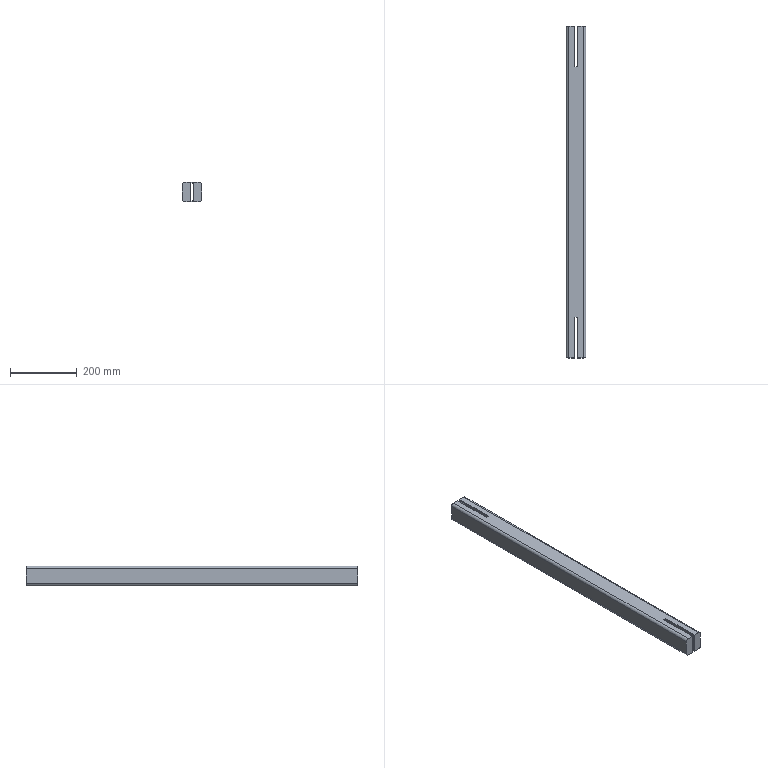Part | SolidWorks | features ICE 3, Extrusion 1 | 1 solid | 32 faces | box 60 x 998 x 60 mm | volume 853297 mm3 | plane 24 | cylinder 8 | commonest cylinder face diameters 8 x4 16 x4
STEP:
#1=CARTESIAN_POINT('',(22.,998.,-30.));
#2=VERTEX_POINT('',#1);
#3=CARTESIAN_POINT('',(4.5,998.,-30.));
#4=VERTEX_POINT('',#3);
#5=CARTESIAN_POINT('',(-22.,998.,-30.));
#6=DIRECTION('',(-1.,0.,0.));
#7=VECTOR('',#6,1000.);
#8=LINE('',#5,#7);
#9=EDGE_CURVE('',#2,#4,#8,.T.);
#10=ORIENTED_EDGE('',*,*,#9,.T.);
#11=CARTESIAN_POINT('',(4.5,998.,30.));
#12=VERTEX_POINT('',#11);
#13=CARTESIAN_POINT('',(4.5,998.,22.));
#14=DIRECTION('',(0.,0.,1.));
#15=VECTOR('',#14,1000.);
#16=LINE('',#13,#15);
#17=EDGE_CURVE('',#4,#12,#16,.T.);
#18=ORIENTED_EDGE('',*,*,#17,.T.);
#19=CARTESIAN_POINT('',(22.,998.,30.));
#20=VERTEX_POINT('',#19);
#21=CARTESIAN_POINT('',(-22.,998.,30.));
#22=DIRECTION('',(1.,0.,0.));
#23=VECTOR('',#22,1000.);
#24=LINE('',#21,#23);
#25=EDGE_CURVE('',#12,#20,#24,.T.);
#26=ORIENTED_EDGE('',*,*,#25,.T.);
#27=CARTESIAN_POINT('',(30.,998.,22.));
#28=VERTEX_POINT('',#27);
#29=CARTESIAN_POINT('',(22.,998.,22.));
#30=DIRECTION('',(0.,1.,0.));
#31=DIRECTION('',(0.,0.,1.));
#32=AXIS2_PLACEMENT_3D('',#29,#30,#31);
#33=CIRCLE('',#32,8.);
#34=EDGE_CURVE('',#20,#28,#33,.T.);
#35=ORIENTED_EDGE('',*,*,#34,.T.);
#36=CARTESIAN_POINT('',(30.,998.,-22.));
#37=VERTEX_POINT('',#36);
#38=CARTESIAN_POINT('',(30.,998.,22.));
#39=DIRECTION('',(0.,0.,-1.));
#40=VECTOR('',#39,1000.);
#41=LINE('',#38,#40);
#42=EDGE_CURVE('',#28,#37,#41,.T.);
#43=ORIENTED_EDGE('',*,*,#42,.T.);
#44=CARTESIAN_POINT('',(22.,998.,-22.));
#45=DIRECTION('',(0.,1.,0.));
#46=DIRECTION('',(0.,0.,-1.));
#47=AXIS2_PLACEMENT_3D('',#44,#45,#46);
#48=CIRCLE('',#47,8.);
#49=EDGE_CURVE('',#37,#2,#48,.T.);
#50=ORIENTED_EDGE('',*,*,#49,.T.);
#51=EDGE_LOOP('',(#10,#18,#26,#35,#43,#50));
#52=FACE_OUTER_BOUND('',#51,.T.);
#53=CARTESIAN_POINT('',(-22.,998.,22.));
#54=DIRECTION('',(0.,-1.,0.));
#55=DIRECTION('',(0.,0.,-1.));
#56=AXIS2_PLACEMENT_3D('',#53,#54,#55);
#57=PLANE('',#56);
#58=ADVANCED_FACE('',(#52),#57,.F.);
#59=CARTESIAN_POINT('',(4.5,0.,30.));
#60=VERTEX_POINT('',#59);
#61=CARTESIAN_POINT('',(22.,0.,30.));
#62=VERTEX_POINT('',#61);
#63=CARTESIAN_POINT('',(-22.,0.,30.));
#64=DIRECTION('',(1.,0.,0.));
#65=VECTOR('',#64,1000.);
#66=LINE('',#63,#65);
#67=EDGE_CURVE('',#60,#62,#66,.T.);
#68=ORIENTED_EDGE('',*,*,#67,.F.);
#69=CARTESIAN_POINT('',(4.5,0.,-30.));
#70=VERTEX_POINT('',#69);
#71=CARTESIAN_POINT('',(4.5,0.,22.));
#72=DIRECTION('',(0.,0.,1.));
#73=VECTOR('',#72,1000.);
#74=LINE('',#71,#73);
#75=EDGE_CURVE('',#70,#60,#74,.T.);
#76=ORIENTED_EDGE('',*,*,#75,.F.);
#77=CARTESIAN_POINT('',(22.,0.,-30.));
#78=VERTEX_POINT('',#77);
#79=CARTESIAN_POINT('',(-22.,0.,-30.));
#80=DIRECTION('',(-1.,0.,0.));
#81=VECTOR('',#80,1000.);
#82=LINE('',#79,#81);
#83=EDGE_CURVE('',#78,#70,#82,.T.);
#84=ORIENTED_EDGE('',*,*,#83,.F.);
#85=CARTESIAN_POINT('',(30.,0.,-22.));
#86=VERTEX_POINT('',#85);
#87=CARTESIAN_POINT('',(22.,0.,-22.));
#88=DIRECTION('',(0.,1.,0.));
#89=DIRECTION('',(0.,0.,-1.));
#90=AXIS2_PLACEMENT_3D('',#87,#88,#89);
#91=CIRCLE('',#90,8.);
#92=EDGE_CURVE('',#86,#78,#91,.T.);
#93=ORIENTED_EDGE('',*,*,#92,.F.);
#94=CARTESIAN_POINT('',(30.,0.,22.));
#95=VERTEX_POINT('',#94);
#96=CARTESIAN_POINT('',(30.,0.,22.));
#97=DIRECTION('',(0.,0.,-1.));
#98=VECTOR('',#97,1000.);
#99=LINE('',#96,#98);
#100=EDGE_CURVE('',#95,#86,#99,.T.);
#101=ORIENTED_EDGE('',*,*,#100,.F.);
#102=CARTESIAN_POINT('',(22.,0.,22.));
#103=DIRECTION('',(0.,1.,0.));
#104=DIRECTION('',(0.,0.,1.));
#105=AXIS2_PLACEMENT_3D('',#102,#103,#104);
#106=CIRCLE('',#105,8.);
#107=EDGE_CURVE('',#62,#95,#106,.T.);
#108=ORIENTED_EDGE('',*,*,#107,.F.);
#109=EDGE_LOOP('',(#68,#76,#84,#93,#101,#108));
#110=FACE_OUTER_BOUND('',#109,.T.);
#111=CARTESIAN_POINT('',(-22.,0.,22.));
#112=DIRECTION('',(0.,-1.,0.));
#113=DIRECTION('',(0.,0.,-1.));
#114=AXIS2_PLACEMENT_3D('',#111,#112,#113);
#115=PLANE('',#114);
#116=ADVANCED_FACE('',(#110),#115,.T.);
#117=CARTESIAN_POINT('',(-4.5,998.,30.));
#118=VERTEX_POINT('',#117);
#119=CARTESIAN_POINT('',(-4.5,998.,-30.));
#120=VERTEX_POINT('',#119);
#121=CARTESIAN_POINT('',(-4.5,998.,22.));
#122=DIRECTION('',(0.,0.,-1.));
#123=VECTOR('',#122,1000.);
#124=LINE('',#121,#123);
#125=EDGE_CURVE('',#118,#120,#124,.T.);
#126=ORIENTED_EDGE('',*,*,#125,.T.);
#127=CARTESIAN_POINT('',(-22.,998.,-30.));
#128=VERTEX_POINT('',#127);
#129=CARTESIAN_POINT('',(-22.,998.,-30.));
#130=DIRECTION('',(-1.,0.,0.));
#131=VECTOR('',#130,1000.);
#132=LINE('',#129,#131);
#133=EDGE_CURVE('',#120,#128,#132,.T.);
#134=ORIENTED_EDGE('',*,*,#133,.T.);
#135=CARTESIAN_POINT('',(-30.,998.,-22.));
#136=VERTEX_POINT('',#135);
#137=CARTESIAN_POINT('',(-22.,998.,-22.));
#138=DIRECTION('',(0.,1.,0.));
#139=DIRECTION('',(0.,0.,-1.));
#140=AXIS2_PLACEMENT_3D('',#137,#138,#139);
#141=CIRCLE('',#140,8.);
#142=EDGE_CURVE('',#128,#136,#141,.T.);
#143=ORIENTED_EDGE('',*,*,#142,.T.);
#144=CARTESIAN_POINT('',(-30.,998.,22.));
#145=VERTEX_POINT('',#144);
#146=CARTESIAN_POINT('',(-30.,998.,22.));
#147=DIRECTION('',(0.,0.,1.));
#148=VECTOR('',#147,1000.);
#149=LINE('',#146,#148);
#150=EDGE_CURVE('',#136,#145,#149,.T.);
#151=ORIENTED_EDGE('',*,*,#150,.T.);
#152=CARTESIAN_POINT('',(-22.,998.,30.));
#153=VERTEX_POINT('',#152);
#154=CARTESIAN_POINT('',(-22.,998.,22.));
#155=DIRECTION('',(0.,1.,0.));
#156=DIRECTION('',(0.,0.,-1.));
#157=AXIS2_PLACEMENT_3D('',#154,#155,#156);
#158=CIRCLE('',#157,8.);
#159=EDGE_CURVE('',#145,#153,#158,.T.);
#160=ORIENTED_EDGE('',*,*,#159,.T.);
#161=CARTESIAN_POINT('',(-22.,998.,30.));
#162=DIRECTION('',(1.,0.,0.));
#163=VECTOR('',#162,1000.);
#164=LINE('',#161,#163);
#165=EDGE_CURVE('',#153,#118,#164,.T.);
#166=ORIENTED_EDGE('',*,*,#165,.T.);
#167=EDGE_LOOP('',(#126,#134,#143,#151,#160,#166));
#168=FACE_OUTER_BOUND('',#167,.T.);
#169=CARTESIAN_POINT('',(-22.,998.,22.));
#170=DIRECTION('',(0.,-1.,0.));
#171=DIRECTION('',(0.,0.,-1.));
#172=AXIS2_PLACEMENT_3D('',#169,#170,#171);
#173=PLANE('',#172);
#174=ADVANCED_FACE('',(#168),#173,.F.);
#175=CARTESIAN_POINT('',(-4.5,0.,-30.));
#176=VERTEX_POINT('',#175);
#177=CARTESIAN_POINT('',(-22.,0.,-30.));
#178=VERTEX_POINT('',#177);
#179=CARTESIAN_POINT('',(-22.,0.,-30.));
#180=DIRECTION('',(-1.,0.,0.));
#181=VECTOR('',#180,1000.);
#182=LINE('',#179,#181);
#183=EDGE_CURVE('',#176,#178,#182,.T.);
#184=ORIENTED_EDGE('',*,*,#183,.F.);
#185=CARTESIAN_POINT('',(-4.5,0.,30.));
#186=VERTEX_POINT('',#185);
#187=CARTESIAN_POINT('',(-4.5,0.,22.));
#188=DIRECTION('',(0.,0.,-1.));
#189=VECTOR('',#188,1000.);
#190=LINE('',#187,#189);
#191=EDGE_CURVE('',#186,#176,#190,.T.);
#192=ORIENTED_EDGE('',*,*,#191,.F.);
#193=CARTESIAN_POINT('',(-22.,0.,30.));
#194=VERTEX_POINT('',#193);
#195=CARTESIAN_POINT('',(-22.,0.,30.));
#196=DIRECTION('',(1.,0.,0.));
#197=VECTOR('',#196,1000.);
#198=LINE('',#195,#197);
#199=EDGE_CURVE('',#194,#186,#198,.T.);
#200=ORIENTED_EDGE('',*,*,#199,.F.);
#201=CARTESIAN_POINT('',(-30.,0.,22.));
#202=VERTEX_POINT('',#201);
#203=CARTESIAN_POINT('',(-22.,0.,22.));
#204=DIRECTION('',(0.,1.,0.));
#205=DIRECTION('',(0.,0.,-1.));
#206=AXIS2_PLACEMENT_3D('',#203,#204,#205);
#207=CIRCLE('',#206,8.);
#208=EDGE_CURVE('',#202,#194,#207,.T.);
#209=ORIENTED_EDGE('',*,*,#208,.F.);
#210=CARTESIAN_POINT('',(-30.,0.,-22.));
#211=VERTEX_POINT('',#210);
#212=CARTESIAN_POINT('',(-30.,0.,22.));
#213=DIRECTION('',(0.,0.,1.));
#214=VECTOR('',#213,1000.);
#215=LINE('',#212,#214);
#216=EDGE_CURVE('',#211,#202,#215,.T.);
#217=ORIENTED_EDGE('',*,*,#216,.F.);
#218=CARTESIAN_POINT('',(-22.,0.,-22.));
#219=DIRECTION('',(0.,1.,0.));
#220=DIRECTION('',(0.,0.,-1.));
#221=AXIS2_PLACEMENT_3D('',#218,#219,#220);
#222=CIRCLE('',#221,8.);
#223=EDGE_CURVE('',#178,#211,#222,.T.);
#224=ORIENTED_EDGE('',*,*,#223,.F.);
#225=EDGE_LOOP('',(#184,#192,#200,#209,#217,#224));
#226=FACE_OUTER_BOUND('',#225,.T.);
#227=CARTESIAN_POINT('',(-22.,0.,22.));
#228=DIRECTION('',(0.,-1.,0.));
#229=DIRECTION('',(0.,0.,-1.));
#230=AXIS2_PLACEMENT_3D('',#227,#228,#229);
#231=PLANE('',#230);
#232=ADVANCED_FACE('',(#226),#231,.T.);
#233=ORIENTED_EDGE('',*,*,#208,.T.);
#234=CARTESIAN_POINT('',(-22.,998.,30.));
#235=DIRECTION('',(0.,-1.,0.));
#236=VECTOR('',#235,1000.);
#237=LINE('',#234,#236);
#238=EDGE_CURVE('',#153,#194,#237,.T.);
#239=ORIENTED_EDGE('',*,*,#238,.F.);
#240=ORIENTED_EDGE('',*,*,#159,.F.);
#241=CARTESIAN_POINT('',(-30.,998.,22.));
#242=DIRECTION('',(0.,-1.,0.));
#243=VECTOR('',#242,1000.);
#244=LINE('',#241,#243);
#245=EDGE_CURVE('',#145,#202,#244,.T.);
#246=ORIENTED_EDGE('',*,*,#245,.T.);
#247=EDGE_LOOP('',(#233,#239,#240,#246));
#248=FACE_OUTER_BOUND('',#247,.T.);
#249=CARTESIAN_POINT('',(-22.,998.,22.));
#250=DIRECTION('',(0.,-1.,0.));
#251=DIRECTION('',(0.,0.,-1.));
#252=AXIS2_PLACEMENT_3D('',#249,#250,#251);
#253=CYLINDRICAL_SURFACE('',#252,8.);
#254=ADVANCED_FACE('',(#248),#253,.T.);
#255=ORIENTED_EDGE('',*,*,#25,.F.);
#256=CARTESIAN_POINT('',(4.5,876.,30.));
#257=VERTEX_POINT('',#256);
#258=CARTESIAN_POINT('',(4.5,998.,30.));
#259=DIRECTION('',(0.,-1.,0.));
#260=VECTOR('',#259,1000.);
#261=LINE('',#258,#260);
#262=EDGE_CURVE('',#12,#257,#261,.T.);
#263=ORIENTED_EDGE('',*,*,#262,.T.);
#264=CARTESIAN_POINT('',(-4.5,876.,30.));
#265=VERTEX_POINT('',#264);
#266=CARTESIAN_POINT('',(-22.,876.,30.));
#267=DIRECTION('',(-1.,0.,0.));
#268=VECTOR('',#267,1000.);
#269=LINE('',#266,#268);
#270=EDGE_CURVE('',#257,#265,#269,.T.);
#271=ORIENTED_EDGE('',*,*,#270,.T.);
#272=CARTESIAN_POINT('',(-4.5,998.,30.));
#273=DIRECTION('',(0.,1.,0.));
#274=VECTOR('',#273,1000.);
#275=LINE('',#272,#274);
#276=EDGE_CURVE('',#265,#118,#275,.T.);
#277=ORIENTED_EDGE('',*,*,#276,.T.);
#278=ORIENTED_EDGE('',*,*,#165,.F.);
#279=ORIENTED_EDGE('',*,*,#238,.T.);
#280=ORIENTED_EDGE('',*,*,#199,.T.);
#281=CARTESIAN_POINT('',(-4.5,122.,30.));
#282=VERTEX_POINT('',#281);
#283=CARTESIAN_POINT('',(-4.5,998.,30.));
#284=DIRECTION('',(0.,1.,0.));
#285=VECTOR('',#284,1000.);
#286=LINE('',#283,#285);
#287=EDGE_CURVE('',#186,#282,#286,.T.);
#288=ORIENTED_EDGE('',*,*,#287,.T.);
#289=CARTESIAN_POINT('',(4.5,122.,30.));
#290=VERTEX_POINT('',#289);
#291=CARTESIAN_POINT('',(-22.,122.,30.));
#292=DIRECTION('',(1.,0.,0.));
#293=VECTOR('',#292,1000.);
#294=LINE('',#291,#293);
#295=EDGE_CURVE('',#282,#290,#294,.T.);
#296=ORIENTED_EDGE('',*,*,#295,.T.);
#297=CARTESIAN_POINT('',(4.5,998.,30.));
#298=DIRECTION('',(0.,-1.,0.));
#299=VECTOR('',#298,1000.);
#300=LINE('',#297,#299);
#301=EDGE_CURVE('',#290,#60,#300,.T.);
#302=ORIENTED_EDGE('',*,*,#301,.T.);
#303=ORIENTED_EDGE('',*,*,#67,.T.);
#304=CARTESIAN_POINT('',(22.,998.,30.));
#305=DIRECTION('',(0.,-1.,0.));
#306=VECTOR('',#305,1000.);
#307=LINE('',#304,#306);
#308=EDGE_CURVE('',#20,#62,#307,.T.);
#309=ORIENTED_EDGE('',*,*,#308,.F.);
#310=EDGE_LOOP('',(#255,#263,#271,#277,#278,#279,#280,#288,#296,#302,#303,#309));
#311=FACE_OUTER_BOUND('',#310,.T.);
#312=CARTESIAN_POINT('',(-22.,998.,30.));
#313=DIRECTION('',(0.,0.,-1.));
#314=DIRECTION('',(-1.,0.,0.));
#315=AXIS2_PLACEMENT_3D('',#312,#313,#314);
#316=PLANE('',#315);
#317=ADVANCED_FACE('',(#311),#316,.F.);
#318=ORIENTED_EDGE('',*,*,#107,.T.);
#319=CARTESIAN_POINT('',(30.,998.,22.));
#320=DIRECTION('',(0.,-1.,0.));
#321=VECTOR('',#320,1000.);
#322=LINE('',#319,#321);
#323=EDGE_CURVE('',#28,#95,#322,.T.);
#324=ORIENTED_EDGE('',*,*,#323,.F.);
#325=ORIENTED_EDGE('',*,*,#34,.F.);
#326=ORIENTED_EDGE('',*,*,#308,.T.);
#327=EDGE_LOOP('',(#318,#324,#325,#326));
#328=FACE_OUTER_BOUND('',#327,.T.);
#329=CARTESIAN_POINT('',(22.,998.,22.));
#330=DIRECTION('',(0.,-1.,0.));
#331=DIRECTION('',(0.,0.,-1.));
#332=AXIS2_PLACEMENT_3D('',#329,#330,#331);
#333=CYLINDRICAL_SURFACE('',#332,8.);
#334=ADVANCED_FACE('',(#328),#333,.T.);
#335=ORIENTED_EDGE('',*,*,#100,.T.);
#336=CARTESIAN_POINT('',(30.,998.,-22.));
#337=DIRECTION('',(0.,-1.,0.));
#338=VECTOR('',#337,1000.);
#339=LINE('',#336,#338);
#340=EDGE_CURVE('',#37,#86,#339,.T.);
#341=ORIENTED_EDGE('',*,*,#340,.F.);
#342=ORIENTED_EDGE('',*,*,#42,.F.);
#343=ORIENTED_EDGE('',*,*,#323,.T.);
#344=EDGE_LOOP('',(#335,#341,#342,#343));
#345=FACE_OUTER_BOUND('',#344,.T.);
#346=CARTESIAN_POINT('',(30.,998.,22.));
#347=DIRECTION('',(-1.,0.,0.));
#348=DIRECTION('',(0.,0.,1.));
#349=AXIS2_PLACEMENT_3D('',#346,#347,#348);
#350=PLANE('',#349);
#351=ADVANCED_FACE('',(#345),#350,.F.);
#352=ORIENTED_EDGE('',*,*,#92,.T.);
#353=CARTESIAN_POINT('',(22.,998.,-30.));
#354=DIRECTION('',(0.,-1.,0.));
#355=VECTOR('',#354,1000.);
#356=LINE('',#353,#355);
#357=EDGE_CURVE('',#2,#78,#356,.T.);
#358=ORIENTED_EDGE('',*,*,#357,.F.);
#359=ORIENTED_EDGE('',*,*,#49,.F.);
#360=ORIENTED_EDGE('',*,*,#340,.T.);
#361=EDGE_LOOP('',(#352,#358,#359,#360));
#362=FACE_OUTER_BOUND('',#361,.T.);
#363=CARTESIAN_POINT('',(22.,998.,-22.));
#364=DIRECTION('',(0.,-1.,0.));
#365=DIRECTION('',(0.,0.,-1.));
#366=AXIS2_PLACEMENT_3D('',#363,#364,#365);
#367=CYLINDRICAL_SURFACE('',#366,8.);
#368=ADVANCED_FACE('',(#362),#367,.T.);
#369=CARTESIAN_POINT('',(-4.5,876.,-30.));
#370=VERTEX_POINT('',#369);
#371=CARTESIAN_POINT('',(4.5,876.,-30.));
#372=VERTEX_POINT('',#371);
#373=CARTESIAN_POINT('',(-4.5,876.,-30.));
#374=DIRECTION('',(1.,0.,0.));
#375=VECTOR('',#374,1000.);
#376=LINE('',#373,#375);
#377=EDGE_CURVE('',#370,#372,#376,.T.);
#378=ORIENTED_EDGE('',*,*,#377,.T.);
#379=CARTESIAN_POINT('',(4.5,1120.,-30.));
#380=DIRECTION('',(0.,1.,0.));
#381=VECTOR('',#380,1000.);
#382=LINE('',#379,#381);
#383=EDGE_CURVE('',#372,#4,#382,.T.);
#384=ORIENTED_EDGE('',*,*,#383,.T.);
#385=ORIENTED_EDGE('',*,*,#9,.F.);
#386=ORIENTED_EDGE('',*,*,#357,.T.);
#387=ORIENTED_EDGE('',*,*,#83,.T.);
#388=CARTESIAN_POINT('',(4.5,122.,-30.));
#389=VERTEX_POINT('',#388);
#390=CARTESIAN_POINT('',(4.5,-122.,-30.));
#391=DIRECTION('',(0.,1.,0.));
#392=VECTOR('',#391,1000.);
#393=LINE('',#390,#392);
#394=EDGE_CURVE('',#70,#389,#393,.T.);
#395=ORIENTED_EDGE('',*,*,#394,.T.);
#396=CARTESIAN_POINT('',(-4.5,122.,-30.));
#397=VERTEX_POINT('',#396);
#398=CARTESIAN_POINT('',(-4.5,122.,-30.));
#399=DIRECTION('',(-1.,0.,0.));
#400=VECTOR('',#399,1000.);
#401=LINE('',#398,#400);
#402=EDGE_CURVE('',#389,#397,#401,.T.);
#403=ORIENTED_EDGE('',*,*,#402,.T.);
#404=CARTESIAN_POINT('',(-4.5,-122.,-30.));
#405=DIRECTION('',(0.,-1.,0.));
#406=VECTOR('',#405,1000.);
#407=LINE('',#404,#406);
#408=EDGE_CURVE('',#397,#176,#407,.T.);
#409=ORIENTED_EDGE('',*,*,#408,.T.);
#410=ORIENTED_EDGE('',*,*,#183,.T.);
#411=CARTESIAN_POINT('',(-22.,998.,-30.));
#412=DIRECTION('',(0.,-1.,0.));
#413=VECTOR('',#412,1000.);
#414=LINE('',#411,#413);
#415=EDGE_CURVE('',#128,#178,#414,.T.);
#416=ORIENTED_EDGE('',*,*,#415,.F.);
#417=ORIENTED_EDGE('',*,*,#133,.F.);
#418=CARTESIAN_POINT('',(-4.5,1120.,-30.));
#419=DIRECTION('',(0.,-1.,0.));
#420=VECTOR('',#419,1000.);
#421=LINE('',#418,#420);
#422=EDGE_CURVE('',#120,#370,#421,.T.);
#423=ORIENTED_EDGE('',*,*,#422,.T.);
#424=EDGE_LOOP('',(#378,#384,#385,#386,#387,#395,#403,#409,#410,#416,#417,#423));
#425=FACE_OUTER_BOUND('',#424,.T.);
#426=CARTESIAN_POINT('',(-22.,998.,-30.));
#427=DIRECTION('',(0.,0.,1.));
#428=DIRECTION('',(1.,0.,0.));
#429=AXIS2_PLACEMENT_3D('',#426,#427,#428);
#430=PLANE('',#429);
#431=ADVANCED_FACE('',(#425),#430,.F.);
#432=ORIENTED_EDGE('',*,*,#223,.T.);
#433=CARTESIAN_POINT('',(-30.,998.,-22.));
#434=DIRECTION('',(0.,-1.,0.));
#435=VECTOR('',#434,1000.);
#436=LINE('',#433,#435);
#437=EDGE_CURVE('',#136,#211,#436,.T.);
#438=ORIENTED_EDGE('',*,*,#437,.F.);
#439=ORIENTED_EDGE('',*,*,#142,.F.);
#440=ORIENTED_EDGE('',*,*,#415,.T.);
#441=EDGE_LOOP('',(#432,#438,#439,#440));
#442=FACE_OUTER_BOUND('',#441,.T.);
#443=CARTESIAN_POINT('',(-22.,998.,-22.));
#444=DIRECTION('',(0.,-1.,0.));
#445=DIRECTION('',(0.,0.,-1.));
#446=AXIS2_PLACEMENT_3D('',#443,#444,#445);
#447=CYLINDRICAL_SURFACE('',#446,8.);
#448=ADVANCED_FACE('',(#442),#447,.T.);
#449=ORIENTED_EDGE('',*,*,#216,.T.);
#450=ORIENTED_EDGE('',*,*,#245,.F.);
#451=ORIENTED_EDGE('',*,*,#150,.F.);
#452=ORIENTED_EDGE('',*,*,#437,.T.);
#453=EDGE_LOOP('',(#449,#450,#451,#452));
#454=FACE_OUTER_BOUND('',#453,.T.);
#455=CARTESIAN_POINT('',(-30.,998.,22.));
#456=DIRECTION('',(1.,0.,0.));
#457=DIRECTION('',(0.,0.,-1.));
#458=AXIS2_PLACEMENT_3D('',#455,#456,#457);
#459=PLANE('',#458);
#460=ADVANCED_FACE('',(#454),#459,.F.);
#461=CARTESIAN_POINT('',(-22.,4.,-26.));
#462=VERTEX_POINT('',#461);
#463=CARTESIAN_POINT('',(-26.,4.,-22.));
#464=VERTEX_POINT('',#463);
#465=CARTESIAN_POINT('',(-22.,4.,-22.));
#466=DIRECTION('',(0.,1.,0.));
#467=DIRECTION('',(0.,0.,1.));
#468=AXIS2_PLACEMENT_3D('',#465,#466,#467);
#469=CIRCLE('',#468,4.);
#470=EDGE_CURVE('',#462,#464,#469,.T.);
#471=ORIENTED_EDGE('',*,*,#470,.F.);
#472=CARTESIAN_POINT('',(-22.,994.,-26.));
#473=VERTEX_POINT('',#472);
#474=CARTESIAN_POINT('',(-22.,998.,-26.));
#475=DIRECTION('',(0.,-1.,0.));
#476=VECTOR('',#475,1000.);
#477=LINE('',#474,#476);
#478=EDGE_CURVE('',#473,#462,#477,.T.);
#479=ORIENTED_EDGE('',*,*,#478,.F.);
#480=CARTESIAN_POINT('',(-26.,994.,-22.));
#481=VERTEX_POINT('',#480);
#482=CARTESIAN_POINT('',(-22.,994.,-22.));
#483=DIRECTION('',(0.,-1.,0.));
#484=DIRECTION('',(0.,0.,-1.));
#485=AXIS2_PLACEMENT_3D('',#482,#483,#484);
#486=CIRCLE('',#485,4.);
#487=EDGE_CURVE('',#481,#473,#486,.T.);
#488=ORIENTED_EDGE('',*,*,#487,.F.);
#489=CARTESIAN_POINT('',(-26.,998.,-22.));
#490=DIRECTION('',(0.,-1.,0.));
#491=VECTOR('',#490,1000.);
#492=LINE('',#489,#491);
#493=EDGE_CURVE('',#481,#464,#492,.T.);
#494=ORIENTED_EDGE('',*,*,#493,.T.);
#495=EDGE_LOOP('',(#471,#479,#488,#494));
#496=FACE_OUTER_BOUND('',#495,.T.);
#497=CARTESIAN_POINT('',(-22.,998.,-22.));
#498=DIRECTION('',(0.,-1.,0.));
#499=DIRECTION('',(0.,0.,-1.));
#500=AXIS2_PLACEMENT_3D('',#497,#498,#499);
#501=CYLINDRICAL_SURFACE('',#500,4.);
#502=ADVANCED_FACE('',(#496),#501,.F.);
#503=CARTESIAN_POINT('',(-26.,4.,22.));
#504=VERTEX_POINT('',#503);
#505=CARTESIAN_POINT('',(-26.,4.,26.));
#506=DIRECTION('',(0.,0.,-1.));
#507=VECTOR('',#506,1000.);
#508=LINE('',#505,#507);
#509=EDGE_CURVE('',#504,#464,#508,.T.);
#510=ORIENTED_EDGE('',*,*,#509,.T.);
#511=ORIENTED_EDGE('',*,*,#493,.F.);
#512=CARTESIAN_POINT('',(-26.,994.,22.));
#513=VERTEX_POINT('',#512);
#514=CARTESIAN_POINT('',(-26.,994.,-26.));
#515=DIRECTION('',(0.,0.,1.));
#516=VECTOR('',#515,1000.);
#517=LINE('',#514,#516);
#518=EDGE_CURVE('',#481,#513,#517,.T.);
#519=ORIENTED_EDGE('',*,*,#518,.T.);
#520=CARTESIAN_POINT('',(-26.,998.,22.));
#521=DIRECTION('',(0.,-1.,0.));
#522=VECTOR('',#521,1000.);
#523=LINE('',#520,#522);
#524=EDGE_CURVE('',#513,#504,#523,.T.);
#525=ORIENTED_EDGE('',*,*,#524,.T.);
#526=EDGE_LOOP('',(#510,#511,#519,#525));
#527=FACE_OUTER_BOUND('',#526,.T.);
#528=CARTESIAN_POINT('',(-26.,998.,22.));
#529=DIRECTION('',(1.,0.,0.));
#530=DIRECTION('',(0.,0.,-1.));
#531=AXIS2_PLACEMENT_3D('',#528,#529,#530);
#532=PLANE('',#531);
#533=ADVANCED_FACE('',(#527),#532,.T.);
#534=CARTESIAN_POINT('',(-22.,4.,26.));
#535=VERTEX_POINT('',#534);
#536=CARTESIAN_POINT('',(-22.,4.,22.));
#537=DIRECTION('',(0.,1.,0.));
#538=DIRECTION('',(0.,0.,1.));
#539=AXIS2_PLACEMENT_3D('',#536,#537,#538);
#540=CIRCLE('',#539,4.);
#541=EDGE_CURVE('',#504,#535,#540,.T.);
#542=ORIENTED_EDGE('',*,*,#541,.F.);
#543=ORIENTED_EDGE('',*,*,#524,.F.);
#544=CARTESIAN_POINT('',(-22.,994.,26.));
#545=VERTEX_POINT('',#544);
#546=CARTESIAN_POINT('',(-22.,994.,22.));
#547=DIRECTION('',(0.,-1.,0.));
#548=DIRECTION('',(0.,0.,-1.));
#549=AXIS2_PLACEMENT_3D('',#546,#547,#548);
#550=CIRCLE('',#549,4.);
#551=EDGE_CURVE('',#545,#513,#550,.T.);
#552=ORIENTED_EDGE('',*,*,#551,.F.);
#553=CARTESIAN_POINT('',(-22.,998.,26.));
#554=DIRECTION('',(0.,-1.,0.));
#555=VECTOR('',#554,1000.);
#556=LINE('',#553,#555);
#557=EDGE_CURVE('',#545,#535,#556,.T.);
#558=ORIENTED_EDGE('',*,*,#557,.T.);
#559=EDGE_LOOP('',(#542,#543,#552,#558));
#560=FACE_OUTER_BOUND('',#559,.T.);
#561=CARTESIAN_POINT('',(-22.,998.,22.));
#562=DIRECTION('',(0.,-1.,0.));
#563=DIRECTION('',(0.,0.,-1.));
#564=AXIS2_PLACEMENT_3D('',#561,#562,#563);
#565=CYLINDRICAL_SURFACE('',#564,4.);
#566=ADVANCED_FACE('',(#560),#565,.F.);
#567=CARTESIAN_POINT('',(22.,4.,26.));
#568=VERTEX_POINT('',#567);
#569=CARTESIAN_POINT('',(4.5,4.,26.));
#570=VERTEX_POINT('',#569);
#571=CARTESIAN_POINT('',(4.5,4.,26.));
#572=DIRECTION('',(-1.,0.,0.));
#573=VECTOR('',#572,1000.);
#574=LINE('',#571,#573);
#575=EDGE_CURVE('',#568,#570,#574,.T.);
#576=ORIENTED_EDGE('',*,*,#575,.T.);
#577=CARTESIAN_POINT('',(4.5,122.,26.));
#578=VERTEX_POINT('',#577);
#579=CARTESIAN_POINT('',(4.5,998.,26.));
#580=DIRECTION('',(0.,-1.,0.));
#581=VECTOR('',#580,1000.);
#582=LINE('',#579,#581);
#583=EDGE_CURVE('',#578,#570,#582,.T.);
#584=ORIENTED_EDGE('',*,*,#583,.F.);
#585=CARTESIAN_POINT('',(-4.5,122.,26.));
#586=VERTEX_POINT('',#585);
#587=CARTESIAN_POINT('',(-22.,122.,26.));
#588=DIRECTION('',(1.,0.,0.));
#589=VECTOR('',#588,1000.);
#590=LINE('',#587,#589);
#591=EDGE_CURVE('',#586,#578,#590,.T.);
#592=ORIENTED_EDGE('',*,*,#591,.F.);
#593=CARTESIAN_POINT('',(-4.5,4.,26.));
#594=VERTEX_POINT('',#593);
#595=CARTESIAN_POINT('',(-4.5,998.,26.));
#596=DIRECTION('',(0.,1.,0.));
#597=VECTOR('',#596,1000.);
#598=LINE('',#595,#597);
#599=EDGE_CURVE('',#594,#586,#598,.T.);
#600=ORIENTED_EDGE('',*,*,#599,.F.);
#601=CARTESIAN_POINT('',(-4.5,4.,26.));
#602=DIRECTION('',(-1.,0.,0.));
#603=VECTOR('',#602,1000.);
#604=LINE('',#601,#603);
#605=EDGE_CURVE('',#594,#535,#604,.T.);
#606=ORIENTED_EDGE('',*,*,#605,.T.);
#607=ORIENTED_EDGE('',*,*,#557,.F.);
#608=CARTESIAN_POINT('',(-4.5,994.,26.));
#609=VERTEX_POINT('',#608);
#610=CARTESIAN_POINT('',(-4.5,994.,26.));
#611=DIRECTION('',(1.,0.,0.));
#612=VECTOR('',#611,1000.);
#613=LINE('',#610,#612);
#614=EDGE_CURVE('',#545,#609,#613,.T.);
#615=ORIENTED_EDGE('',*,*,#614,.T.);
#616=CARTESIAN_POINT('',(-4.5,876.,26.));
#617=VERTEX_POINT('',#616);
#618=CARTESIAN_POINT('',(-4.5,998.,26.));
#619=DIRECTION('',(0.,1.,0.));
#620=VECTOR('',#619,1000.);
#621=LINE('',#618,#620);
#622=EDGE_CURVE('',#617,#609,#621,.T.);
#623=ORIENTED_EDGE('',*,*,#622,.F.);
#624=CARTESIAN_POINT('',(4.5,876.,26.));
#625=VERTEX_POINT('',#624);
#626=CARTESIAN_POINT('',(-22.,876.,26.));
#627=DIRECTION('',(-1.,0.,0.));
#628=VECTOR('',#627,1000.);
#629=LINE('',#626,#628);
#630=EDGE_CURVE('',#625,#617,#629,.T.);
#631=ORIENTED_EDGE('',*,*,#630,.F.);
#632=CARTESIAN_POINT('',(4.5,994.,26.));
#633=VERTEX_POINT('',#632);
#634=CARTESIAN_POINT('',(4.5,998.,26.));
#635=DIRECTION('',(0.,-1.,0.));
#636=VECTOR('',#635,1000.);
#637=LINE('',#634,#636);
#638=EDGE_CURVE('',#633,#625,#637,.T.);
#639=ORIENTED_EDGE('',*,*,#638,.F.);
#640=CARTESIAN_POINT('',(22.,994.,26.));
#641=VERTEX_POINT('',#640);
#642=CARTESIAN_POINT('',(4.5,994.,26.));
#643=DIRECTION('',(1.,0.,0.));
#644=VECTOR('',#643,1000.);
#645=LINE('',#642,#644);
#646=EDGE_CURVE('',#633,#641,#645,.T.);
#647=ORIENTED_EDGE('',*,*,#646,.T.);
#648=CARTESIAN_POINT('',(22.,998.,26.));
#649=DIRECTION('',(0.,-1.,0.));
#650=VECTOR('',#649,1000.);
#651=LINE('',#648,#650);
#652=EDGE_CURVE('',#641,#568,#651,.T.);
#653=ORIENTED_EDGE('',*,*,#652,.T.);
#654=EDGE_LOOP('',(#576,#584,#592,#600,#606,#607,#615,#623,#631,#639,#647,#653));
#655=FACE_OUTER_BOUND('',#654,.T.);
#656=CARTESIAN_POINT('',(-22.,998.,26.));
#657=DIRECTION('',(0.,0.,-1.));
#658=DIRECTION('',(-1.,0.,0.));
#659=AXIS2_PLACEMENT_3D('',#656,#657,#658);
#660=PLANE('',#659);
#661=ADVANCED_FACE('',(#655),#660,.T.);
#662=CARTESIAN_POINT('',(26.,4.,22.));
#663=VERTEX_POINT('',#662);
#664=CARTESIAN_POINT('',(22.,4.,22.));
#665=DIRECTION('',(0.,1.,0.));
#666=DIRECTION('',(0.,0.,1.));
#667=AXIS2_PLACEMENT_3D('',#664,#665,#666);
#668=CIRCLE('',#667,4.);
#669=EDGE_CURVE('',#568,#663,#668,.T.);
#670=ORIENTED_EDGE('',*,*,#669,.F.);
#671=ORIENTED_EDGE('',*,*,#652,.F.);
#672=CARTESIAN_POINT('',(26.,994.,22.));
#673=VERTEX_POINT('',#672);
#674=CARTESIAN_POINT('',(22.,994.,22.));
#675=DIRECTION('',(0.,-1.,0.));
#676=DIRECTION('',(0.,0.,-1.));
#677=AXIS2_PLACEMENT_3D('',#674,#675,#676);
#678=CIRCLE('',#677,4.);
#679=EDGE_CURVE('',#673,#641,#678,.T.);
#680=ORIENTED_EDGE('',*,*,#679,.F.);
#681=CARTESIAN_POINT('',(26.,998.,22.));
#682=DIRECTION('',(0.,-1.,0.));
#683=VECTOR('',#682,1000.);
#684=LINE('',#681,#683);
#685=EDGE_CURVE('',#673,#663,#684,.T.);
#686=ORIENTED_EDGE('',*,*,#685,.T.);
#687=EDGE_LOOP('',(#670,#671,#680,#686));
#688=FACE_OUTER_BOUND('',#687,.T.);
#689=CARTESIAN_POINT('',(22.,998.,22.));
#690=DIRECTION('',(0.,-1.,0.));
#691=DIRECTION('',(0.,0.,-1.));
#692=AXIS2_PLACEMENT_3D('',#689,#690,#691);
#693=CYLINDRICAL_SURFACE('',#692,4.);
#694=ADVANCED_FACE('',(#688),#693,.F.);
#695=CARTESIAN_POINT('',(26.,4.,-22.));
#696=VERTEX_POINT('',#695);
#697=CARTESIAN_POINT('',(26.,4.,26.));
#698=DIRECTION('',(0.,0.,1.));
#699=VECTOR('',#698,1000.);
#700=LINE('',#697,#699);
#701=EDGE_CURVE('',#696,#663,#700,.T.);
#702=ORIENTED_EDGE('',*,*,#701,.T.);
#703=ORIENTED_EDGE('',*,*,#685,.F.);
#704=CARTESIAN_POINT('',(26.,994.,-22.));
#705=VERTEX_POINT('',#704);
#706=CARTESIAN_POINT('',(26.,994.,-26.));
#707=DIRECTION('',(0.,0.,-1.));
#708=VECTOR('',#707,1000.);
#709=LINE('',#706,#708);
#710=EDGE_CURVE('',#673,#705,#709,.T.);
#711=ORIENTED_EDGE('',*,*,#710,.T.);
#712=CARTESIAN_POINT('',(26.,998.,-22.));
#713=DIRECTION('',(0.,-1.,0.));
#714=VECTOR('',#713,1000.);
#715=LINE('',#712,#714);
#716=EDGE_CURVE('',#705,#696,#715,.T.);
#717=ORIENTED_EDGE('',*,*,#716,.T.);
#718=EDGE_LOOP('',(#702,#703,#711,#717));
#719=FACE_OUTER_BOUND('',#718,.T.);
#720=CARTESIAN_POINT('',(26.,998.,22.));
#721=DIRECTION('',(-1.,0.,0.));
#722=DIRECTION('',(0.,0.,1.));
#723=AXIS2_PLACEMENT_3D('',#720,#721,#722);
#724=PLANE('',#723);
#725=ADVANCED_FACE('',(#719),#724,.T.);
#726=CARTESIAN_POINT('',(22.,4.,-26.));
#727=VERTEX_POINT('',#726);
#728=CARTESIAN_POINT('',(22.,4.,-22.));
#729=DIRECTION('',(0.,1.,0.));
#730=DIRECTION('',(0.,0.,1.));
#731=AXIS2_PLACEMENT_3D('',#728,#729,#730);
#732=CIRCLE('',#731,4.);
#733=EDGE_CURVE('',#696,#727,#732,.T.);
#734=ORIENTED_EDGE('',*,*,#733,.F.);
#735=ORIENTED_EDGE('',*,*,#716,.F.);
#736=CARTESIAN_POINT('',(22.,994.,-26.));
#737=VERTEX_POINT('',#736);
#738=CARTESIAN_POINT('',(22.,994.,-22.));
#739=DIRECTION('',(0.,-1.,0.));
#740=DIRECTION('',(0.,0.,-1.));
#741=AXIS2_PLACEMENT_3D('',#738,#739,#740);
#742=CIRCLE('',#741,4.);
#743=EDGE_CURVE('',#737,#705,#742,.T.);
#744=ORIENTED_EDGE('',*,*,#743,.F.);
#745=CARTESIAN_POINT('',(22.,998.,-26.));
#746=DIRECTION('',(0.,-1.,0.));
#747=VECTOR('',#746,1000.);
#748=LINE('',#745,#747);
#749=EDGE_CURVE('',#737,#727,#748,.T.);
#750=ORIENTED_EDGE('',*,*,#749,.T.);
#751=EDGE_LOOP('',(#734,#735,#744,#750));
#752=FACE_OUTER_BOUND('',#751,.T.);
#753=CARTESIAN_POINT('',(22.,998.,-22.));
#754=DIRECTION('',(0.,-1.,0.));
#755=DIRECTION('',(0.,0.,-1.));
#756=AXIS2_PLACEMENT_3D('',#753,#754,#755);
#757=CYLINDRICAL_SURFACE('',#756,4.);
#758=ADVANCED_FACE('',(#752),#757,.F.);
#759=CARTESIAN_POINT('',(4.5,4.,-26.));
#760=VERTEX_POINT('',#759);
#761=CARTESIAN_POINT('',(4.5,4.,-26.));
#762=DIRECTION('',(1.,0.,0.));
#763=VECTOR('',#762,1000.);
#764=LINE('',#761,#763);
#765=EDGE_CURVE('',#760,#727,#764,.T.);
#766=ORIENTED_EDGE('',*,*,#765,.T.);
#767=ORIENTED_EDGE('',*,*,#749,.F.);
#768=CARTESIAN_POINT('',(4.5,994.,-26.));
#769=VERTEX_POINT('',#768);
#770=CARTESIAN_POINT('',(4.5,994.,-26.));
#771=DIRECTION('',(-1.,0.,0.));
#772=VECTOR('',#771,1000.);
#773=LINE('',#770,#772);
#774=EDGE_CURVE('',#737,#769,#773,.T.);
#775=ORIENTED_EDGE('',*,*,#774,.T.);
#776=CARTESIAN_POINT('',(4.5,876.,-26.));
#777=VERTEX_POINT('',#776);
#778=CARTESIAN_POINT('',(4.5,998.,-26.));
#779=DIRECTION('',(0.,1.,0.));
#780=VECTOR('',#779,1000.);
#781=LINE('',#778,#780);
#782=EDGE_CURVE('',#777,#769,#781,.T.);
#783=ORIENTED_EDGE('',*,*,#782,.F.);
#784=CARTESIAN_POINT('',(-4.5,876.,-26.));
#785=VERTEX_POINT('',#784);
#786=CARTESIAN_POINT('',(-22.,876.,-26.));
#787=DIRECTION('',(1.,0.,0.));
#788=VECTOR('',#787,1000.);
#789=LINE('',#786,#788);
#790=EDGE_CURVE('',#785,#777,#789,.T.);
#791=ORIENTED_EDGE('',*,*,#790,.F.);
#792=CARTESIAN_POINT('',(-4.5,994.,-26.));
#793=VERTEX_POINT('',#792);
#794=CARTESIAN_POINT('',(-4.5,998.,-26.));
#795=DIRECTION('',(0.,-1.,0.));
#796=VECTOR('',#795,1000.);
#797=LINE('',#794,#796);
#798=EDGE_CURVE('',#793,#785,#797,.T.);
#799=ORIENTED_EDGE('',*,*,#798,.F.);
#800=CARTESIAN_POINT('',(-4.5,994.,-26.));
#801=DIRECTION('',(-1.,0.,0.));
#802=VECTOR('',#801,1000.);
#803=LINE('',#800,#802);
#804=EDGE_CURVE('',#793,#473,#803,.T.);
#805=ORIENTED_EDGE('',*,*,#804,.T.);
#806=ORIENTED_EDGE('',*,*,#478,.T.);
#807=CARTESIAN_POINT('',(-4.5,4.,-26.));
#808=VERTEX_POINT('',#807);
#809=CARTESIAN_POINT('',(-4.5,4.,-26.));
#810=DIRECTION('',(1.,0.,0.));
#811=VECTOR('',#810,1000.);
#812=LINE('',#809,#811);
#813=EDGE_CURVE('',#462,#808,#812,.T.);
#814=ORIENTED_EDGE('',*,*,#813,.T.);
#815=CARTESIAN_POINT('',(-4.5,122.,-26.));
#816=VERTEX_POINT('',#815);
#817=CARTESIAN_POINT('',(-4.5,998.,-26.));
#818=DIRECTION('',(0.,-1.,0.));
#819=VECTOR('',#818,1000.);
#820=LINE('',#817,#819);
#821=EDGE_CURVE('',#816,#808,#820,.T.);
#822=ORIENTED_EDGE('',*,*,#821,.F.);
#823=CARTESIAN_POINT('',(4.5,122.,-26.));
#824=VERTEX_POINT('',#823);
#825=CARTESIAN_POINT('',(-22.,122.,-26.));
#826=DIRECTION('',(-1.,0.,0.));
#827=VECTOR('',#826,1000.);
#828=LINE('',#825,#827);
#829=EDGE_CURVE('',#824,#816,#828,.T.);
#830=ORIENTED_EDGE('',*,*,#829,.F.);
#831=CARTESIAN_POINT('',(4.5,998.,-26.));
#832=DIRECTION('',(0.,1.,0.));
#833=VECTOR('',#832,1000.);
#834=LINE('',#831,#833);
#835=EDGE_CURVE('',#760,#824,#834,.T.);
#836=ORIENTED_EDGE('',*,*,#835,.F.);
#837=EDGE_LOOP('',(#766,#767,#775,#783,#791,#799,#805,#806,#814,#822,#830,#836));
#838=FACE_OUTER_BOUND('',#837,.T.);
#839=CARTESIAN_POINT('',(-22.,998.,-26.));
#840=DIRECTION('',(0.,0.,1.));
#841=DIRECTION('',(1.,0.,0.));
#842=AXIS2_PLACEMENT_3D('',#839,#840,#841);
#843=PLANE('',#842);
#844=ADVANCED_FACE('',(#838),#843,.T.);
#845=ORIENTED_EDGE('',*,*,#829,.T.);
#846=CARTESIAN_POINT('',(-4.5,122.,-30.));
#847=DIRECTION('',(0.,0.,1.));
#848=VECTOR('',#847,1000.);
#849=LINE('',#846,#848);
#850=EDGE_CURVE('',#397,#816,#849,.T.);
#851=ORIENTED_EDGE('',*,*,#850,.F.);
#852=ORIENTED_EDGE('',*,*,#402,.F.);
#853=CARTESIAN_POINT('',(4.5,122.,-30.));
#854=DIRECTION('',(0.,0.,1.));
#855=VECTOR('',#854,1000.);
#856=LINE('',#853,#855);
#857=EDGE_CURVE('',#389,#824,#856,.T.);
#858=ORIENTED_EDGE('',*,*,#857,.T.);
#859=EDGE_LOOP('',(#845,#851,#852,#858));
#860=FACE_OUTER_BOUND('',#859,.T.);
#861=CARTESIAN_POINT('',(-4.5,122.,-30.));
#862=DIRECTION('',(0.,1.,0.));
#863=DIRECTION('',(0.,0.,1.));
#864=AXIS2_PLACEMENT_3D('',#861,#862,#863);
#865=PLANE('',#864);
#866=ADVANCED_FACE('',(#860),#865,.F.);
#867=ORIENTED_EDGE('',*,*,#790,.T.);
#868=CARTESIAN_POINT('',(4.5,876.,-30.));
#869=DIRECTION('',(0.,0.,1.));
#870=VECTOR('',#869,1000.);
#871=LINE('',#868,#870);
#872=EDGE_CURVE('',#372,#777,#871,.T.);
#873=ORIENTED_EDGE('',*,*,#872,.F.);
#874=ORIENTED_EDGE('',*,*,#377,.F.);
#875=CARTESIAN_POINT('',(-4.5,876.,-30.));
#876=DIRECTION('',(0.,0.,1.));
#877=VECTOR('',#876,1000.);
#878=LINE('',#875,#877);
#879=EDGE_CURVE('',#370,#785,#878,.T.);
#880=ORIENTED_EDGE('',*,*,#879,.T.);
#881=EDGE_LOOP('',(#867,#873,#874,#880));
#882=FACE_OUTER_BOUND('',#881,.T.);
#883=CARTESIAN_POINT('',(-4.5,876.,-30.));
#884=DIRECTION('',(0.,-1.,0.));
#885=DIRECTION('',(0.,0.,-1.));
#886=AXIS2_PLACEMENT_3D('',#883,#884,#885);
#887=PLANE('',#886);
#888=ADVANCED_FACE('',(#882),#887,.F.);
#889=CARTESIAN_POINT('',(4.5,122.,-30.));
#890=DIRECTION('',(0.,0.,1.));
#891=VECTOR('',#890,1000.);
#892=LINE('',#889,#891);
#893=EDGE_CURVE('',#578,#290,#892,.T.);
#894=ORIENTED_EDGE('',*,*,#893,.F.);
#895=ORIENTED_EDGE('',*,*,#583,.T.);
#896=CARTESIAN_POINT('',(4.5,4.,26.));
#897=DIRECTION('',(0.,0.,-1.));
#898=VECTOR('',#897,1000.);
#899=LINE('',#896,#898);
#900=EDGE_CURVE('',#570,#760,#899,.T.);
#901=ORIENTED_EDGE('',*,*,#900,.T.);
#902=ORIENTED_EDGE('',*,*,#835,.T.);
#903=ORIENTED_EDGE('',*,*,#857,.F.);
#904=ORIENTED_EDGE('',*,*,#394,.F.);
#905=ORIENTED_EDGE('',*,*,#75,.T.);
#906=ORIENTED_EDGE('',*,*,#301,.F.);
#907=EDGE_LOOP('',(#894,#895,#901,#902,#903,#904,#905,#906));
#908=FACE_OUTER_BOUND('',#907,.T.);
#909=CARTESIAN_POINT('',(4.5,-122.,-30.));
#910=DIRECTION('',(1.,0.,0.));
#911=DIRECTION('',(0.,0.,-1.));
#912=AXIS2_PLACEMENT_3D('',#909,#910,#911);
#913=PLANE('',#912);
#914=ADVANCED_FACE('',(#908),#913,.F.);
#915=ORIENTED_EDGE('',*,*,#191,.T.);
#916=ORIENTED_EDGE('',*,*,#408,.F.);
#917=ORIENTED_EDGE('',*,*,#850,.T.);
#918=ORIENTED_EDGE('',*,*,#821,.T.);
#919=CARTESIAN_POINT('',(-4.5,4.,26.));
#920=DIRECTION('',(0.,0.,1.));
#921=VECTOR('',#920,1000.);
#922=LINE('',#919,#921);
#923=EDGE_CURVE('',#808,#594,#922,.T.);
#924=ORIENTED_EDGE('',*,*,#923,.T.);
#925=ORIENTED_EDGE('',*,*,#599,.T.);
#926=CARTESIAN_POINT('',(-4.5,122.,-30.));
#927=DIRECTION('',(0.,0.,1.));
#928=VECTOR('',#927,1000.);
#929=LINE('',#926,#928);
#930=EDGE_CURVE('',#586,#282,#929,.T.);
#931=ORIENTED_EDGE('',*,*,#930,.T.);
#932=ORIENTED_EDGE('',*,*,#287,.F.);
#933=EDGE_LOOP('',(#915,#916,#917,#918,#924,#925,#931,#932));
#934=FACE_OUTER_BOUND('',#933,.T.);
#935=CARTESIAN_POINT('',(-4.5,-122.,-30.));
#936=DIRECTION('',(-1.,0.,0.));
#937=DIRECTION('',(0.,0.,1.));
#938=AXIS2_PLACEMENT_3D('',#935,#936,#937);
#939=PLANE('',#938);
#940=ADVANCED_FACE('',(#934),#939,.F.);
#941=ORIENTED_EDGE('',*,*,#930,.F.);
#942=ORIENTED_EDGE('',*,*,#591,.T.);
#943=ORIENTED_EDGE('',*,*,#893,.T.);
#944=ORIENTED_EDGE('',*,*,#295,.F.);
#945=EDGE_LOOP('',(#941,#942,#943,#944));
#946=FACE_OUTER_BOUND('',#945,.T.);
#947=CARTESIAN_POINT('',(-4.5,122.,-30.));
#948=DIRECTION('',(0.,1.,0.));
#949=DIRECTION('',(0.,0.,1.));
#950=AXIS2_PLACEMENT_3D('',#947,#948,#949);
#951=PLANE('',#950);
#952=ADVANCED_FACE('',(#946),#951,.F.);
#953=ORIENTED_EDGE('',*,*,#17,.F.);
#954=ORIENTED_EDGE('',*,*,#383,.F.);
#955=ORIENTED_EDGE('',*,*,#872,.T.);
#956=ORIENTED_EDGE('',*,*,#782,.T.);
#957=CARTESIAN_POINT('',(4.5,994.,-26.));
#958=DIRECTION('',(0.,0.,1.));
#959=VECTOR('',#958,1000.);
#960=LINE('',#957,#959);
#961=EDGE_CURVE('',#769,#633,#960,.T.);
#962=ORIENTED_EDGE('',*,*,#961,.T.);
#963=ORIENTED_EDGE('',*,*,#638,.T.);
#964=CARTESIAN_POINT('',(4.5,876.,-30.));
#965=DIRECTION('',(0.,0.,1.));
#966=VECTOR('',#965,1000.);
#967=LINE('',#964,#966);
#968=EDGE_CURVE('',#625,#257,#967,.T.);
#969=ORIENTED_EDGE('',*,*,#968,.T.);
#970=ORIENTED_EDGE('',*,*,#262,.F.);
#971=EDGE_LOOP('',(#953,#954,#955,#956,#962,#963,#969,#970));
#972=FACE_OUTER_BOUND('',#971,.T.);
#973=CARTESIAN_POINT('',(4.5,1120.,-30.));
#974=DIRECTION('',(1.,0.,0.));
#975=DIRECTION('',(0.,0.,-1.));
#976=AXIS2_PLACEMENT_3D('',#973,#974,#975);
#977=PLANE('',#976);
#978=ADVANCED_FACE('',(#972),#977,.F.);
#979=ORIENTED_EDGE('',*,*,#968,.F.);
#980=ORIENTED_EDGE('',*,*,#630,.T.);
#981=CARTESIAN_POINT('',(-4.5,876.,-30.));
#982=DIRECTION('',(0.,0.,1.));
#983=VECTOR('',#982,1000.);
#984=LINE('',#981,#983);
#985=EDGE_CURVE('',#617,#265,#984,.T.);
#986=ORIENTED_EDGE('',*,*,#985,.T.);
#987=ORIENTED_EDGE('',*,*,#270,.F.);
#988=EDGE_LOOP('',(#979,#980,#986,#987));
#989=FACE_OUTER_BOUND('',#988,.T.);
#990=CARTESIAN_POINT('',(-4.5,876.,-30.));
#991=DIRECTION('',(0.,-1.,0.));
#992=DIRECTION('',(0.,0.,-1.));
#993=AXIS2_PLACEMENT_3D('',#990,#991,#992);
#994=PLANE('',#993);
#995=ADVANCED_FACE('',(#989),#994,.F.);
#996=ORIENTED_EDGE('',*,*,#985,.F.);
#997=ORIENTED_EDGE('',*,*,#622,.T.);
#998=CARTESIAN_POINT('',(-4.5,994.,-26.));
#999=DIRECTION('',(0.,0.,-1.));
#1000=VECTOR('',#999,1000.);
#1001=LINE('',#998,#1000);
#1002=EDGE_CURVE('',#609,#793,#1001,.T.);
#1003=ORIENTED_EDGE('',*,*,#1002,.T.);
#1004=ORIENTED_EDGE('',*,*,#798,.T.);
#1005=ORIENTED_EDGE('',*,*,#879,.F.);
#1006=ORIENTED_EDGE('',*,*,#422,.F.);
#1007=ORIENTED_EDGE('',*,*,#125,.F.);
#1008=ORIENTED_EDGE('',*,*,#276,.F.);
#1009=EDGE_LOOP('',(#996,#997,#1003,#1004,#1005,#1006,#1007,#1008));
#1010=FACE_OUTER_BOUND('',#1009,.T.);
#1011=CARTESIAN_POINT('',(-4.5,1120.,-30.));
#1012=DIRECTION('',(-1.,0.,0.));
#1013=DIRECTION('',(0.,0.,1.));
#1014=AXIS2_PLACEMENT_3D('',#1011,#1012,#1013);
#1015=PLANE('',#1014);
#1016=ADVANCED_FACE('',(#1010),#1015,.F.);
#1017=ORIENTED_EDGE('',*,*,#518,.F.);
#1018=ORIENTED_EDGE('',*,*,#487,.T.);
#1019=ORIENTED_EDGE('',*,*,#804,.F.);
#1020=ORIENTED_EDGE('',*,*,#1002,.F.);
#1021=ORIENTED_EDGE('',*,*,#614,.F.);
#1022=ORIENTED_EDGE('',*,*,#551,.T.);
#1023=EDGE_LOOP('',(#1017,#1018,#1019,#1020,#1021,#1022));
#1024=FACE_OUTER_BOUND('',#1023,.T.);
#1025=CARTESIAN_POINT('',(0.,994.,0.));
#1026=DIRECTION('',(0.,-1.,0.));
#1027=DIRECTION('',(0.,0.,-1.));
#1028=AXIS2_PLACEMENT_3D('',#1025,#1026,#1027);
#1029=PLANE('',#1028);
#1030=ADVANCED_FACE('',(#1024),#1029,.T.);
#1031=ORIENTED_EDGE('',*,*,#710,.F.);
#1032=ORIENTED_EDGE('',*,*,#679,.T.);
#1033=ORIENTED_EDGE('',*,*,#646,.F.);
#1034=ORIENTED_EDGE('',*,*,#961,.F.);
#1035=ORIENTED_EDGE('',*,*,#774,.F.);
#1036=ORIENTED_EDGE('',*,*,#743,.T.);
#1037=EDGE_LOOP('',(#1031,#1032,#1033,#1034,#1035,#1036));
#1038=FACE_OUTER_BOUND('',#1037,.T.);
#1039=CARTESIAN_POINT('',(0.,994.,0.));
#1040=DIRECTION('',(0.,-1.,0.));
#1041=DIRECTION('',(0.,0.,-1.));
#1042=AXIS2_PLACEMENT_3D('',#1039,#1040,#1041);
#1043=PLANE('',#1042);
#1044=ADVANCED_FACE('',(#1038),#1043,.T.);
#1045=ORIENTED_EDGE('',*,*,#813,.F.);
#1046=ORIENTED_EDGE('',*,*,#470,.T.);
#1047=ORIENTED_EDGE('',*,*,#509,.F.);
#1048=ORIENTED_EDGE('',*,*,#541,.T.);
#1049=ORIENTED_EDGE('',*,*,#605,.F.);
#1050=ORIENTED_EDGE('',*,*,#923,.F.);
#1051=EDGE_LOOP('',(#1045,#1046,#1047,#1048,#1049,#1050));
#1052=FACE_OUTER_BOUND('',#1051,.T.);
#1053=CARTESIAN_POINT('',(0.,4.,0.));
#1054=DIRECTION('',(0.,1.,0.));
#1055=DIRECTION('',(0.,0.,1.));
#1056=AXIS2_PLACEMENT_3D('',#1053,#1054,#1055);
#1057=PLANE('',#1056);
#1058=ADVANCED_FACE('',(#1052),#1057,.T.);
#1059=ORIENTED_EDGE('',*,*,#575,.F.);
#1060=ORIENTED_EDGE('',*,*,#669,.T.);
#1061=ORIENTED_EDGE('',*,*,#701,.F.);
#1062=ORIENTED_EDGE('',*,*,#733,.T.);
#1063=ORIENTED_EDGE('',*,*,#765,.F.);
#1064=ORIENTED_EDGE('',*,*,#900,.F.);
#1065=EDGE_LOOP('',(#1059,#1060,#1061,#1062,#1063,#1064));
#1066=FACE_OUTER_BOUND('',#1065,.T.);
#1067=CARTESIAN_POINT('',(0.,4.,0.));
#1068=DIRECTION('',(0.,1.,0.));
#1069=DIRECTION('',(0.,0.,1.));
#1070=AXIS2_PLACEMENT_3D('',#1067,#1068,#1069);
#1071=PLANE('',#1070);
#1072=ADVANCED_FACE('',(#1066),#1071,.T.);
#1073=CLOSED_SHELL('',(#58,#116,#174,#232,#254,#317,#334,#351,#368,#431,#448,#460,#502,#533,#566,#661,#694,#725,#758,#844,#866,#888,#914,#940,#952,#978,#995,#1016,#1030,#1044,#1058,#1072));
#1074=MANIFOLD_SOLID_BREP('',#1073);
#1075=CARTESIAN_POINT('',(0.,0.,0.));
#1076=DIRECTION('',(0.,0.,1.));
#1077=DIRECTION('',(1.,0.,0.));
#1078=AXIS2_PLACEMENT_3D('',#1075,#1076,#1077);
#1079=(LENGTH_UNIT()NAMED_UNIT(*)SI_UNIT(.MILLI.,.METRE.));
#1080=UNCERTAINTY_MEASURE_WITH_UNIT(LENGTH_MEASURE(0.00001),#1079,'','');
#1081=(NAMED_UNIT(*)PLANE_ANGLE_UNIT()SI_UNIT($,.RADIAN.));
#1082=(NAMED_UNIT(*)SI_UNIT($,.STERADIAN.)SOLID_ANGLE_UNIT());
#1083=(GEOMETRIC_REPRESENTATION_CONTEXT(3)GLOBAL_UNCERTAINTY_ASSIGNED_CONTEXT((#1080))GLOBAL_UNIT_ASSIGNED_CONTEXT((#1079,#1081,#1082))REPRESENTATION_CONTEXT('',''));
#1084=ADVANCED_BREP_SHAPE_REPRESENTATION('',(#1074,#1078),#1083);